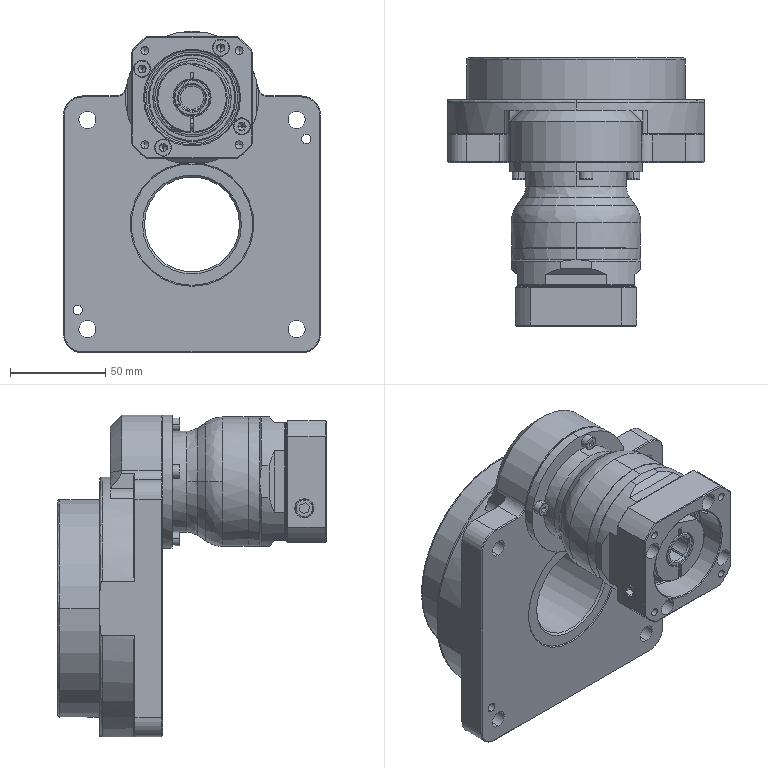Part | SolidWorks | features BaseBody 2 | 2 solids | 898 faces | box 135 x 141 x 169.1 mm | volume 931698 mm3 | plane 321 | cylinder 264 | cone 261 | spline 52 | commonest cylinder face diameters 4.2 x42 5 x18 9 x17 4.5 x16 3.3 x14 5.5 x10